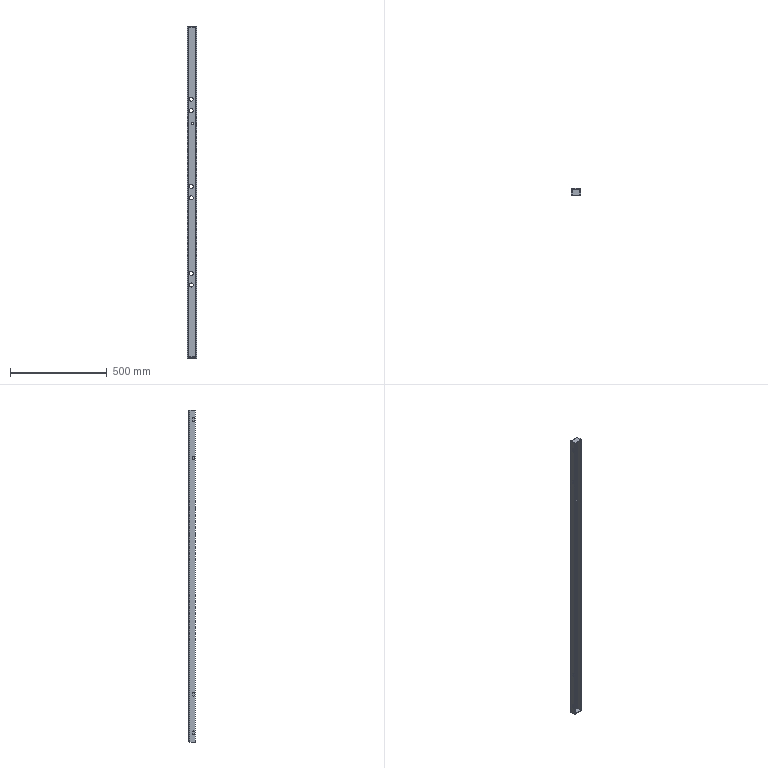Part | STEP file | SYL_0392D6J1SYL0380DJ10-1310194 | 1 solid | 76 faces | box 50 x 35 x 1715 mm | volume 736400 mm3 | cylinder 38 | plane 30 | spline 8 | commonest cylinder face diameters 10 x16 21 x12 6 x4 14 x4 12 x2